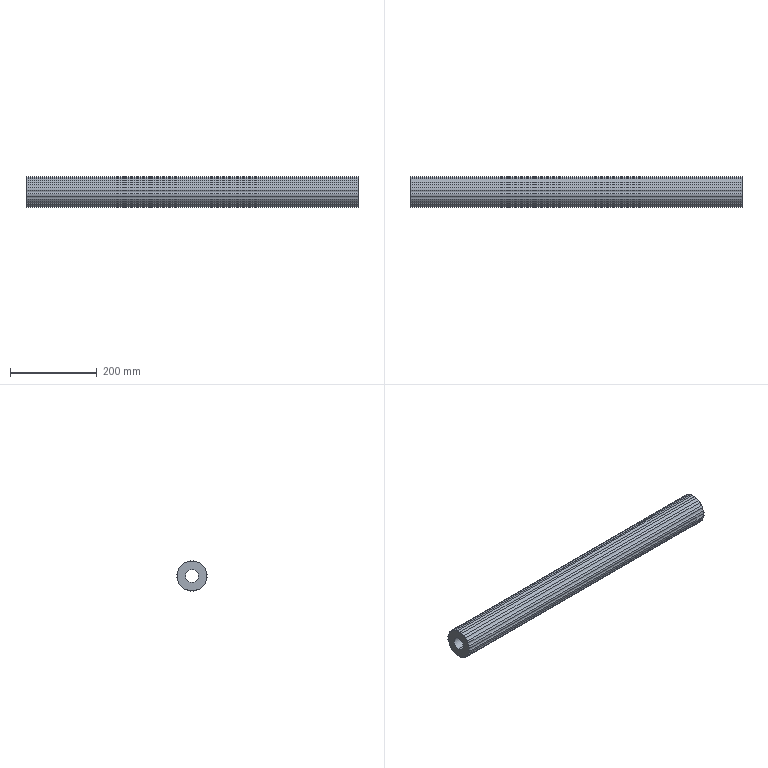Part | SolidWorks | features CirPattern 1, Extrusion 1, ICE 1 | 1 solid | 39 faces | box 767 x 69.535 x 69.535 mm | volume 2311745 mm3 | cylinder 37 | plane 2 | commonest cylinder face diameters 14.407 x19 70 x16 30 x2
STEP:
#1=CARTESIAN_POINT('',(767.,-15.591,-30.436));
#2=VERTEX_POINT('',#1);
#3=CARTESIAN_POINT('',(767.,-9.585,-33.662));
#4=VERTEX_POINT('',#3);
#5=CARTESIAN_POINT('',(767.,-15.591,-37.64));
#6=DIRECTION('',(-1.,0.,0.));
#7=DIRECTION('',(0.,0.9239,-0.3827));
#8=AXIS2_PLACEMENT_3D('',#5,#6,#7);
#9=CIRCLE('',#8,7.203);
#10=EDGE_CURVE('',#2,#4,#9,.T.);
#11=ORIENTED_EDGE('',*,*,#10,.F.);
#12=CARTESIAN_POINT('',(0.,-15.591,-30.436));
#13=VERTEX_POINT('',#12);
#14=CARTESIAN_POINT('',(767.,-15.591,-30.436));
#15=DIRECTION('',(-1.,0.,0.));
#16=VECTOR('',#15,1000.);
#17=LINE('',#14,#16);
#18=EDGE_CURVE('',#2,#13,#17,.T.);
#19=ORIENTED_EDGE('',*,*,#18,.T.);
#20=CARTESIAN_POINT('',(0.,-9.585,-33.662));
#21=VERTEX_POINT('',#20);
#22=CARTESIAN_POINT('',(0.,-15.591,-37.64));
#23=DIRECTION('',(-1.,0.,0.));
#24=DIRECTION('',(0.,0.9239,-0.3827));
#25=AXIS2_PLACEMENT_3D('',#22,#23,#24);
#26=CIRCLE('',#25,7.203);
#27=EDGE_CURVE('',#13,#21,#26,.T.);
#28=ORIENTED_EDGE('',*,*,#27,.T.);
#29=CARTESIAN_POINT('',(383.5,-9.585,-33.662));
#30=DIRECTION('',(-1.,0.,0.));
#31=VECTOR('',#30,1000.);
#32=LINE('',#29,#31);
#33=EDGE_CURVE('',#4,#21,#32,.T.);
#34=ORIENTED_EDGE('',*,*,#33,.F.);
#35=EDGE_LOOP('',(#11,#19,#28,#34));
#36=FACE_OUTER_BOUND('',#35,.T.);
#37=CARTESIAN_POINT('',(767.,-15.591,-37.64));
#38=DIRECTION('',(-1.,0.,0.));
#39=DIRECTION('',(0.,0.,1.));
#40=AXIS2_PLACEMENT_3D('',#37,#38,#39);
#41=CYLINDRICAL_SURFACE('',#40,7.203);
#42=ADVANCED_FACE('',(#36),#41,.F.);
#43=CARTESIAN_POINT('',(767.,15.591,-30.436));
#44=VERTEX_POINT('',#43);
#45=CARTESIAN_POINT('',(767.,17.025,-30.58));
#46=VERTEX_POINT('',#45);
#47=CARTESIAN_POINT('',(767.,15.591,-37.64));
#48=DIRECTION('',(-1.,0.,0.));
#49=DIRECTION('',(0.,0.9239,0.3827));
#50=AXIS2_PLACEMENT_3D('',#47,#48,#49);
#51=CIRCLE('',#50,7.203);
#52=EDGE_CURVE('',#44,#46,#51,.T.);
#53=ORIENTED_EDGE('',*,*,#52,.F.);
#54=CARTESIAN_POINT('',(0.,15.591,-30.436));
#55=VERTEX_POINT('',#54);
#56=CARTESIAN_POINT('',(767.,15.591,-30.436));
#57=DIRECTION('',(-1.,0.,0.));
#58=VECTOR('',#57,1000.);
#59=LINE('',#56,#58);
#60=EDGE_CURVE('',#44,#55,#59,.T.);
#61=ORIENTED_EDGE('',*,*,#60,.T.);
#62=CARTESIAN_POINT('',(0.,17.025,-30.58));
#63=VERTEX_POINT('',#62);
#64=CARTESIAN_POINT('',(0.,15.591,-37.64));
#65=DIRECTION('',(-1.,0.,0.));
#66=DIRECTION('',(0.,0.9239,0.3827));
#67=AXIS2_PLACEMENT_3D('',#64,#65,#66);
#68=CIRCLE('',#67,7.203);
#69=EDGE_CURVE('',#55,#63,#68,.T.);
#70=ORIENTED_EDGE('',*,*,#69,.T.);
#71=CARTESIAN_POINT('',(383.5,17.025,-30.58));
#72=DIRECTION('',(-1.,0.,0.));
#73=VECTOR('',#72,1000.);
#74=LINE('',#71,#73);
#75=EDGE_CURVE('',#46,#63,#74,.T.);
#76=ORIENTED_EDGE('',*,*,#75,.F.);
#77=EDGE_LOOP('',(#53,#61,#70,#76));
#78=FACE_OUTER_BOUND('',#77,.T.);
#79=CARTESIAN_POINT('',(767.,15.591,-37.64));
#80=DIRECTION('',(-1.,0.,0.));
#81=DIRECTION('',(0.,0.,1.));
#82=AXIS2_PLACEMENT_3D('',#79,#80,#81);
#83=CYLINDRICAL_SURFACE('',#82,7.203);
#84=ADVANCED_FACE('',(#78),#83,.F.);
#85=CARTESIAN_POINT('',(767.,0.,-33.537));
#86=VERTEX_POINT('',#85);
#87=CARTESIAN_POINT('',(767.,4.026,-34.768));
#88=VERTEX_POINT('',#87);
#89=CARTESIAN_POINT('',(767.,0.,-40.741));
#90=DIRECTION('',(-1.,0.,0.));
#91=DIRECTION('',(0.,1.,0.));
#92=AXIS2_PLACEMENT_3D('',#89,#90,#91);
#93=CIRCLE('',#92,7.203);
#94=EDGE_CURVE('',#86,#88,#93,.T.);
#95=ORIENTED_EDGE('',*,*,#94,.F.);
#96=CARTESIAN_POINT('',(0.,0.,-33.537));
#97=VERTEX_POINT('',#96);
#98=CARTESIAN_POINT('',(767.,0.,-33.537));
#99=DIRECTION('',(-1.,0.,0.));
#100=VECTOR('',#99,1000.);
#101=LINE('',#98,#100);
#102=EDGE_CURVE('',#86,#97,#101,.T.);
#103=ORIENTED_EDGE('',*,*,#102,.T.);
#104=CARTESIAN_POINT('',(0.,4.026,-34.768));
#105=VERTEX_POINT('',#104);
#106=CARTESIAN_POINT('',(0.,0.,-40.741));
#107=DIRECTION('',(-1.,0.,0.));
#108=DIRECTION('',(0.,1.,0.));
#109=AXIS2_PLACEMENT_3D('',#106,#107,#108);
#110=CIRCLE('',#109,7.203);
#111=EDGE_CURVE('',#97,#105,#110,.T.);
#112=ORIENTED_EDGE('',*,*,#111,.T.);
#113=CARTESIAN_POINT('',(383.5,4.026,-34.768));
#114=DIRECTION('',(-1.,0.,0.));
#115=VECTOR('',#114,1000.);
#116=LINE('',#113,#115);
#117=EDGE_CURVE('',#88,#105,#116,.T.);
#118=ORIENTED_EDGE('',*,*,#117,.F.);
#119=EDGE_LOOP('',(#95,#103,#112,#118));
#120=FACE_OUTER_BOUND('',#119,.T.);
#121=CARTESIAN_POINT('',(767.,0.,-40.741));
#122=DIRECTION('',(-1.,0.,0.));
#123=DIRECTION('',(0.,0.,1.));
#124=AXIS2_PLACEMENT_3D('',#121,#122,#123);
#125=CYLINDRICAL_SURFACE('',#124,7.203);
#126=ADVANCED_FACE('',(#120),#125,.F.);
#127=CARTESIAN_POINT('',(767.,0.,15.));
#128=VERTEX_POINT('',#127);
#129=CARTESIAN_POINT('',(767.,0.,-15.));
#130=VERTEX_POINT('',#129);
#131=CARTESIAN_POINT('',(767.,0.,0.));
#132=DIRECTION('',(1.,0.,0.));
#133=DIRECTION('',(0.,0.,-1.));
#134=AXIS2_PLACEMENT_3D('',#131,#132,#133);
#135=CIRCLE('',#134,15.);
#136=EDGE_CURVE('',#128,#130,#135,.T.);
#137=ORIENTED_EDGE('',*,*,#136,.T.);
#138=CARTESIAN_POINT('',(0.,0.,-15.));
#139=VERTEX_POINT('',#138);
#140=CARTESIAN_POINT('',(767.,0.,-15.));
#141=DIRECTION('',(-1.,0.,0.));
#142=VECTOR('',#141,1000.);
#143=LINE('',#140,#142);
#144=EDGE_CURVE('',#130,#139,#143,.T.);
#145=ORIENTED_EDGE('',*,*,#144,.T.);
#146=CARTESIAN_POINT('',(0.,0.,15.));
#147=VERTEX_POINT('',#146);
#148=CARTESIAN_POINT('',(0.,0.,0.));
#149=DIRECTION('',(1.,0.,0.));
#150=DIRECTION('',(0.,0.,-1.));
#151=AXIS2_PLACEMENT_3D('',#148,#149,#150);
#152=CIRCLE('',#151,15.);
#153=EDGE_CURVE('',#147,#139,#152,.T.);
#154=ORIENTED_EDGE('',*,*,#153,.F.);
#155=CARTESIAN_POINT('',(767.,0.,15.));
#156=DIRECTION('',(-1.,0.,0.));
#157=VECTOR('',#156,1000.);
#158=LINE('',#155,#157);
#159=EDGE_CURVE('',#128,#147,#158,.T.);
#160=ORIENTED_EDGE('',*,*,#159,.F.);
#161=EDGE_LOOP('',(#137,#145,#154,#160));
#162=FACE_OUTER_BOUND('',#161,.T.);
#163=CARTESIAN_POINT('',(767.,0.,0.));
#164=DIRECTION('',(-1.,0.,0.));
#165=DIRECTION('',(0.,0.,1.));
#166=AXIS2_PLACEMENT_3D('',#163,#164,#165);
#167=CYLINDRICAL_SURFACE('',#166,15.);
#168=ADVANCED_FACE('',(#162),#167,.F.);
#169=CARTESIAN_POINT('',(0.,9.585,33.662));
#170=VERTEX_POINT('',#169);
#171=CARTESIAN_POINT('',(0.,4.026,34.768));
#172=VERTEX_POINT('',#171);
#173=CARTESIAN_POINT('',(0.,0.,0.));
#174=DIRECTION('',(1.,0.,0.));
#175=DIRECTION('',(0.,0.,-1.));
#176=AXIS2_PLACEMENT_3D('',#173,#174,#175);
#177=CIRCLE('',#176,35.);
#178=EDGE_CURVE('',#170,#172,#177,.T.);
#179=ORIENTED_EDGE('',*,*,#178,.T.);
#180=CARTESIAN_POINT('',(767.,4.026,34.768));
#181=VERTEX_POINT('',#180);
#182=CARTESIAN_POINT('',(383.5,4.026,34.768));
#183=DIRECTION('',(1.,0.,0.));
#184=VECTOR('',#183,1000.);
#185=LINE('',#182,#184);
#186=EDGE_CURVE('',#172,#181,#185,.T.);
#187=ORIENTED_EDGE('',*,*,#186,.T.);
#188=CARTESIAN_POINT('',(767.,9.585,33.662));
#189=VERTEX_POINT('',#188);
#190=CARTESIAN_POINT('',(767.,0.,0.));
#191=DIRECTION('',(1.,0.,0.));
#192=DIRECTION('',(0.,0.,-1.));
#193=AXIS2_PLACEMENT_3D('',#190,#191,#192);
#194=CIRCLE('',#193,35.);
#195=EDGE_CURVE('',#189,#181,#194,.T.);
#196=ORIENTED_EDGE('',*,*,#195,.F.);
#197=CARTESIAN_POINT('',(383.5,9.585,33.662));
#198=DIRECTION('',(-1.,0.,0.));
#199=VECTOR('',#198,1000.);
#200=LINE('',#197,#199);
#201=EDGE_CURVE('',#189,#170,#200,.T.);
#202=ORIENTED_EDGE('',*,*,#201,.T.);
#203=EDGE_LOOP('',(#179,#187,#196,#202));
#204=FACE_OUTER_BOUND('',#203,.T.);
#205=CARTESIAN_POINT('',(767.,0.,0.));
#206=DIRECTION('',(-1.,0.,0.));
#207=DIRECTION('',(0.,0.,1.));
#208=AXIS2_PLACEMENT_3D('',#205,#206,#207);
#209=CYLINDRICAL_SURFACE('',#208,35.);
#210=ADVANCED_FACE('',(#204),#209,.T.);
#211=CARTESIAN_POINT('',(0.,21.737,27.431));
#212=VERTEX_POINT('',#211);
#213=CARTESIAN_POINT('',(0.,17.025,30.58));
#214=VERTEX_POINT('',#213);
#215=CARTESIAN_POINT('',(0.,0.,0.));
#216=DIRECTION('',(1.,0.,0.));
#217=DIRECTION('',(0.,0.,-1.));
#218=AXIS2_PLACEMENT_3D('',#215,#216,#217);
#219=CIRCLE('',#218,35.);
#220=EDGE_CURVE('',#212,#214,#219,.T.);
#221=ORIENTED_EDGE('',*,*,#220,.T.);
#222=CARTESIAN_POINT('',(767.,17.025,30.58));
#223=VERTEX_POINT('',#222);
#224=CARTESIAN_POINT('',(383.5,17.025,30.58));
#225=DIRECTION('',(1.,0.,0.));
#226=VECTOR('',#225,1000.);
#227=LINE('',#224,#226);
#228=EDGE_CURVE('',#214,#223,#227,.T.);
#229=ORIENTED_EDGE('',*,*,#228,.T.);
#230=CARTESIAN_POINT('',(767.,21.737,27.431));
#231=VERTEX_POINT('',#230);
#232=CARTESIAN_POINT('',(767.,0.,0.));
#233=DIRECTION('',(1.,0.,0.));
#234=DIRECTION('',(0.,0.,-1.));
#235=AXIS2_PLACEMENT_3D('',#232,#233,#234);
#236=CIRCLE('',#235,35.);
#237=EDGE_CURVE('',#231,#223,#236,.T.);
#238=ORIENTED_EDGE('',*,*,#237,.F.);
#239=CARTESIAN_POINT('',(383.5,21.737,27.431));
#240=DIRECTION('',(-1.,0.,0.));
#241=VECTOR('',#240,1000.);
#242=LINE('',#239,#241);
#243=EDGE_CURVE('',#231,#212,#242,.T.);
#244=ORIENTED_EDGE('',*,*,#243,.T.);
#245=EDGE_LOOP('',(#221,#229,#238,#244));
#246=FACE_OUTER_BOUND('',#245,.T.);
#247=CARTESIAN_POINT('',(767.,0.,0.));
#248=DIRECTION('',(-1.,0.,0.));
#249=DIRECTION('',(0.,0.,1.));
#250=AXIS2_PLACEMENT_3D('',#247,#248,#249);
#251=CYLINDRICAL_SURFACE('',#250,35.);
#252=ADVANCED_FACE('',(#246),#251,.T.);
#253=CARTESIAN_POINT('',(0.,30.58,17.025));
#254=VERTEX_POINT('',#253);
#255=CARTESIAN_POINT('',(0.,27.431,21.737));
#256=VERTEX_POINT('',#255);
#257=CARTESIAN_POINT('',(0.,0.,0.));
#258=DIRECTION('',(1.,0.,0.));
#259=DIRECTION('',(0.,0.,-1.));
#260=AXIS2_PLACEMENT_3D('',#257,#258,#259);
#261=CIRCLE('',#260,35.);
#262=EDGE_CURVE('',#254,#256,#261,.T.);
#263=ORIENTED_EDGE('',*,*,#262,.T.);
#264=CARTESIAN_POINT('',(767.,27.431,21.737));
#265=VERTEX_POINT('',#264);
#266=CARTESIAN_POINT('',(383.5,27.431,21.737));
#267=DIRECTION('',(1.,0.,0.));
#268=VECTOR('',#267,1000.);
#269=LINE('',#266,#268);
#270=EDGE_CURVE('',#256,#265,#269,.T.);
#271=ORIENTED_EDGE('',*,*,#270,.T.);
#272=CARTESIAN_POINT('',(767.,30.58,17.025));
#273=VERTEX_POINT('',#272);
#274=CARTESIAN_POINT('',(767.,0.,0.));
#275=DIRECTION('',(1.,0.,0.));
#276=DIRECTION('',(0.,0.,-1.));
#277=AXIS2_PLACEMENT_3D('',#274,#275,#276);
#278=CIRCLE('',#277,35.);
#279=EDGE_CURVE('',#273,#265,#278,.T.);
#280=ORIENTED_EDGE('',*,*,#279,.F.);
#281=CARTESIAN_POINT('',(383.5,30.58,17.025));
#282=DIRECTION('',(-1.,0.,0.));
#283=VECTOR('',#282,1000.);
#284=LINE('',#281,#283);
#285=EDGE_CURVE('',#273,#254,#284,.T.);
#286=ORIENTED_EDGE('',*,*,#285,.T.);
#287=EDGE_LOOP('',(#263,#271,#280,#286));
#288=FACE_OUTER_BOUND('',#287,.T.);
#289=CARTESIAN_POINT('',(767.,0.,0.));
#290=DIRECTION('',(-1.,0.,0.));
#291=DIRECTION('',(0.,0.,1.));
#292=AXIS2_PLACEMENT_3D('',#289,#290,#291);
#293=CYLINDRICAL_SURFACE('',#292,35.);
#294=ADVANCED_FACE('',(#288),#293,.T.);
#295=CARTESIAN_POINT('',(0.,-33.662,9.585));
#296=VERTEX_POINT('',#295);
#297=CARTESIAN_POINT('',(0.,-34.768,4.026));
#298=VERTEX_POINT('',#297);
#299=CARTESIAN_POINT('',(0.,0.,0.));
#300=DIRECTION('',(1.,0.,0.));
#301=DIRECTION('',(0.,0.,-1.));
#302=AXIS2_PLACEMENT_3D('',#299,#300,#301);
#303=CIRCLE('',#302,35.);
#304=EDGE_CURVE('',#296,#298,#303,.T.);
#305=ORIENTED_EDGE('',*,*,#304,.T.);
#306=CARTESIAN_POINT('',(767.,-34.768,4.026));
#307=VERTEX_POINT('',#306);
#308=CARTESIAN_POINT('',(383.5,-34.768,4.026));
#309=DIRECTION('',(1.,0.,0.));
#310=VECTOR('',#309,1000.);
#311=LINE('',#308,#310);
#312=EDGE_CURVE('',#298,#307,#311,.T.);
#313=ORIENTED_EDGE('',*,*,#312,.T.);
#314=CARTESIAN_POINT('',(767.,-33.662,9.585));
#315=VERTEX_POINT('',#314);
#316=CARTESIAN_POINT('',(767.,0.,0.));
#317=DIRECTION('',(1.,0.,0.));
#318=DIRECTION('',(0.,0.,-1.));
#319=AXIS2_PLACEMENT_3D('',#316,#317,#318);
#320=CIRCLE('',#319,35.);
#321=EDGE_CURVE('',#315,#307,#320,.T.);
#322=ORIENTED_EDGE('',*,*,#321,.F.);
#323=CARTESIAN_POINT('',(383.5,-33.662,9.585));
#324=DIRECTION('',(-1.,0.,0.));
#325=VECTOR('',#324,1000.);
#326=LINE('',#323,#325);
#327=EDGE_CURVE('',#315,#296,#326,.T.);
#328=ORIENTED_EDGE('',*,*,#327,.T.);
#329=EDGE_LOOP('',(#305,#313,#322,#328));
#330=FACE_OUTER_BOUND('',#329,.T.);
#331=CARTESIAN_POINT('',(767.,0.,0.));
#332=DIRECTION('',(-1.,0.,0.));
#333=DIRECTION('',(0.,0.,1.));
#334=AXIS2_PLACEMENT_3D('',#331,#332,#333);
#335=CYLINDRICAL_SURFACE('',#334,35.);
#336=ADVANCED_FACE('',(#330),#335,.T.);
#337=CARTESIAN_POINT('',(0.,-27.431,21.737));
#338=VERTEX_POINT('',#337);
#339=CARTESIAN_POINT('',(0.,-30.58,17.025));
#340=VERTEX_POINT('',#339);
#341=CARTESIAN_POINT('',(0.,0.,0.));
#342=DIRECTION('',(1.,0.,0.));
#343=DIRECTION('',(0.,0.,-1.));
#344=AXIS2_PLACEMENT_3D('',#341,#342,#343);
#345=CIRCLE('',#344,35.);
#346=EDGE_CURVE('',#338,#340,#345,.T.);
#347=ORIENTED_EDGE('',*,*,#346,.T.);
#348=CARTESIAN_POINT('',(767.,-30.58,17.025));
#349=VERTEX_POINT('',#348);
#350=CARTESIAN_POINT('',(383.5,-30.58,17.025));
#351=DIRECTION('',(1.,0.,0.));
#352=VECTOR('',#351,1000.);
#353=LINE('',#350,#352);
#354=EDGE_CURVE('',#340,#349,#353,.T.);
#355=ORIENTED_EDGE('',*,*,#354,.T.);
#356=CARTESIAN_POINT('',(767.,-27.431,21.737));
#357=VERTEX_POINT('',#356);
#358=CARTESIAN_POINT('',(767.,0.,0.));
#359=DIRECTION('',(1.,0.,0.));
#360=DIRECTION('',(0.,0.,-1.));
#361=AXIS2_PLACEMENT_3D('',#358,#359,#360);
#362=CIRCLE('',#361,35.);
#363=EDGE_CURVE('',#357,#349,#362,.T.);
#364=ORIENTED_EDGE('',*,*,#363,.F.);
#365=CARTESIAN_POINT('',(383.5,-27.431,21.737));
#366=DIRECTION('',(-1.,0.,0.));
#367=VECTOR('',#366,1000.);
#368=LINE('',#365,#367);
#369=EDGE_CURVE('',#357,#338,#368,.T.);
#370=ORIENTED_EDGE('',*,*,#369,.T.);
#371=EDGE_LOOP('',(#347,#355,#364,#370));
#372=FACE_OUTER_BOUND('',#371,.T.);
#373=CARTESIAN_POINT('',(767.,0.,0.));
#374=DIRECTION('',(-1.,0.,0.));
#375=DIRECTION('',(0.,0.,1.));
#376=AXIS2_PLACEMENT_3D('',#373,#374,#375);
#377=CYLINDRICAL_SURFACE('',#376,35.);
#378=ADVANCED_FACE('',(#372),#377,.T.);
#379=CARTESIAN_POINT('',(767.,-4.026,34.768));
#380=VERTEX_POINT('',#379);
#381=CARTESIAN_POINT('',(767.,-9.585,33.662));
#382=VERTEX_POINT('',#381);
#383=CARTESIAN_POINT('',(767.,0.,0.));
#384=DIRECTION('',(1.,0.,0.));
#385=DIRECTION('',(0.,0.,-1.));
#386=AXIS2_PLACEMENT_3D('',#383,#384,#385);
#387=CIRCLE('',#386,35.);
#388=EDGE_CURVE('',#380,#382,#387,.T.);
#389=ORIENTED_EDGE('',*,*,#388,.F.);
#390=CARTESIAN_POINT('',(0.,-4.026,34.768));
#391=VERTEX_POINT('',#390);
#392=CARTESIAN_POINT('',(383.5,-4.026,34.768));
#393=DIRECTION('',(-1.,0.,0.));
#394=VECTOR('',#393,1000.);
#395=LINE('',#392,#394);
#396=EDGE_CURVE('',#380,#391,#395,.T.);
#397=ORIENTED_EDGE('',*,*,#396,.T.);
#398=CARTESIAN_POINT('',(0.,-9.585,33.662));
#399=VERTEX_POINT('',#398);
#400=CARTESIAN_POINT('',(0.,0.,0.));
#401=DIRECTION('',(1.,0.,0.));
#402=DIRECTION('',(0.,0.,-1.));
#403=AXIS2_PLACEMENT_3D('',#400,#401,#402);
#404=CIRCLE('',#403,35.);
#405=EDGE_CURVE('',#391,#399,#404,.T.);
#406=ORIENTED_EDGE('',*,*,#405,.T.);
#407=CARTESIAN_POINT('',(383.5,-9.585,33.662));
#408=DIRECTION('',(1.,0.,0.));
#409=VECTOR('',#408,1000.);
#410=LINE('',#407,#409);
#411=EDGE_CURVE('',#399,#382,#410,.T.);
#412=ORIENTED_EDGE('',*,*,#411,.T.);
#413=EDGE_LOOP('',(#389,#397,#406,#412));
#414=FACE_OUTER_BOUND('',#413,.T.);
#415=CARTESIAN_POINT('',(767.,0.,0.));
#416=DIRECTION('',(-1.,0.,0.));
#417=DIRECTION('',(0.,0.,1.));
#418=AXIS2_PLACEMENT_3D('',#415,#416,#417);
#419=CYLINDRICAL_SURFACE('',#418,35.);
#420=ADVANCED_FACE('',(#414),#419,.T.);
#421=CARTESIAN_POINT('',(767.,-17.025,30.58));
#422=VERTEX_POINT('',#421);
#423=CARTESIAN_POINT('',(767.,-21.737,27.431));
#424=VERTEX_POINT('',#423);
#425=CARTESIAN_POINT('',(767.,0.,0.));
#426=DIRECTION('',(1.,0.,0.));
#427=DIRECTION('',(0.,0.,-1.));
#428=AXIS2_PLACEMENT_3D('',#425,#426,#427);
#429=CIRCLE('',#428,35.);
#430=EDGE_CURVE('',#422,#424,#429,.T.);
#431=ORIENTED_EDGE('',*,*,#430,.F.);
#432=CARTESIAN_POINT('',(0.,-17.025,30.58));
#433=VERTEX_POINT('',#432);
#434=CARTESIAN_POINT('',(383.5,-17.025,30.58));
#435=DIRECTION('',(-1.,0.,0.));
#436=VECTOR('',#435,1000.);
#437=LINE('',#434,#436);
#438=EDGE_CURVE('',#422,#433,#437,.T.);
#439=ORIENTED_EDGE('',*,*,#438,.T.);
#440=CARTESIAN_POINT('',(0.,-21.737,27.431));
#441=VERTEX_POINT('',#440);
#442=CARTESIAN_POINT('',(0.,0.,0.));
#443=DIRECTION('',(1.,0.,0.));
#444=DIRECTION('',(0.,0.,-1.));
#445=AXIS2_PLACEMENT_3D('',#442,#443,#444);
#446=CIRCLE('',#445,35.);
#447=EDGE_CURVE('',#433,#441,#446,.T.);
#448=ORIENTED_EDGE('',*,*,#447,.T.);
#449=CARTESIAN_POINT('',(383.5,-21.737,27.431));
#450=DIRECTION('',(1.,0.,0.));
#451=VECTOR('',#450,1000.);
#452=LINE('',#449,#451);
#453=EDGE_CURVE('',#441,#424,#452,.T.);
#454=ORIENTED_EDGE('',*,*,#453,.T.);
#455=EDGE_LOOP('',(#431,#439,#448,#454));
#456=FACE_OUTER_BOUND('',#455,.T.);
#457=CARTESIAN_POINT('',(767.,0.,0.));
#458=DIRECTION('',(-1.,0.,0.));
#459=DIRECTION('',(0.,0.,1.));
#460=AXIS2_PLACEMENT_3D('',#457,#458,#459);
#461=CYLINDRICAL_SURFACE('',#460,35.);
#462=ADVANCED_FACE('',(#456),#461,.T.);
#463=CARTESIAN_POINT('',(0.,-30.58,-17.025));
#464=VERTEX_POINT('',#463);
#465=CARTESIAN_POINT('',(0.,-27.431,-21.737));
#466=VERTEX_POINT('',#465);
#467=CARTESIAN_POINT('',(0.,0.,0.));
#468=DIRECTION('',(1.,0.,0.));
#469=DIRECTION('',(0.,0.,-1.));
#470=AXIS2_PLACEMENT_3D('',#467,#468,#469);
#471=CIRCLE('',#470,35.);
#472=EDGE_CURVE('',#464,#466,#471,.T.);
#473=ORIENTED_EDGE('',*,*,#472,.T.);
#474=CARTESIAN_POINT('',(767.,-27.431,-21.737));
#475=VERTEX_POINT('',#474);
#476=CARTESIAN_POINT('',(383.5,-27.431,-21.737));
#477=DIRECTION('',(1.,0.,0.));
#478=VECTOR('',#477,1000.);
#479=LINE('',#476,#478);
#480=EDGE_CURVE('',#466,#475,#479,.T.);
#481=ORIENTED_EDGE('',*,*,#480,.T.);
#482=CARTESIAN_POINT('',(767.,-30.58,-17.025));
#483=VERTEX_POINT('',#482);
#484=CARTESIAN_POINT('',(767.,0.,0.));
#485=DIRECTION('',(1.,0.,0.));
#486=DIRECTION('',(0.,0.,-1.));
#487=AXIS2_PLACEMENT_3D('',#484,#485,#486);
#488=CIRCLE('',#487,35.);
#489=EDGE_CURVE('',#483,#475,#488,.T.);
#490=ORIENTED_EDGE('',*,*,#489,.F.);
#491=CARTESIAN_POINT('',(383.5,-30.58,-17.025));
#492=DIRECTION('',(-1.,0.,0.));
#493=VECTOR('',#492,1000.);
#494=LINE('',#491,#493);
#495=EDGE_CURVE('',#483,#464,#494,.T.);
#496=ORIENTED_EDGE('',*,*,#495,.T.);
#497=EDGE_LOOP('',(#473,#481,#490,#496));
#498=FACE_OUTER_BOUND('',#497,.T.);
#499=CARTESIAN_POINT('',(767.,0.,0.));
#500=DIRECTION('',(-1.,0.,0.));
#501=DIRECTION('',(0.,0.,1.));
#502=AXIS2_PLACEMENT_3D('',#499,#500,#501);
#503=CYLINDRICAL_SURFACE('',#502,35.);
#504=ADVANCED_FACE('',(#498),#503,.T.);
#505=CARTESIAN_POINT('',(767.,-21.737,-27.431));
#506=VERTEX_POINT('',#505);
#507=CARTESIAN_POINT('',(767.,-17.025,-30.58));
#508=VERTEX_POINT('',#507);
#509=CARTESIAN_POINT('',(767.,0.,0.));
#510=DIRECTION('',(1.,0.,0.));
#511=DIRECTION('',(0.,0.,-1.));
#512=AXIS2_PLACEMENT_3D('',#509,#510,#511);
#513=CIRCLE('',#512,35.);
#514=EDGE_CURVE('',#506,#508,#513,.T.);
#515=ORIENTED_EDGE('',*,*,#514,.F.);
#516=CARTESIAN_POINT('',(0.,-21.737,-27.431));
#517=VERTEX_POINT('',#516);
#518=CARTESIAN_POINT('',(383.5,-21.737,-27.431));
#519=DIRECTION('',(-1.,0.,0.));
#520=VECTOR('',#519,1000.);
#521=LINE('',#518,#520);
#522=EDGE_CURVE('',#506,#517,#521,.T.);
#523=ORIENTED_EDGE('',*,*,#522,.T.);
#524=CARTESIAN_POINT('',(0.,-17.025,-30.58));
#525=VERTEX_POINT('',#524);
#526=CARTESIAN_POINT('',(0.,0.,0.));
#527=DIRECTION('',(1.,0.,0.));
#528=DIRECTION('',(0.,0.,-1.));
#529=AXIS2_PLACEMENT_3D('',#526,#527,#528);
#530=CIRCLE('',#529,35.);
#531=EDGE_CURVE('',#517,#525,#530,.T.);
#532=ORIENTED_EDGE('',*,*,#531,.T.);
#533=CARTESIAN_POINT('',(383.5,-17.025,-30.58));
#534=DIRECTION('',(1.,0.,0.));
#535=VECTOR('',#534,1000.);
#536=LINE('',#533,#535);
#537=EDGE_CURVE('',#525,#508,#536,.T.);
#538=ORIENTED_EDGE('',*,*,#537,.T.);
#539=EDGE_LOOP('',(#515,#523,#532,#538));
#540=FACE_OUTER_BOUND('',#539,.T.);
#541=CARTESIAN_POINT('',(767.,0.,0.));
#542=DIRECTION('',(-1.,0.,0.));
#543=DIRECTION('',(0.,0.,1.));
#544=AXIS2_PLACEMENT_3D('',#541,#542,#543);
#545=CYLINDRICAL_SURFACE('',#544,35.);
#546=ADVANCED_FACE('',(#540),#545,.T.);
#547=CARTESIAN_POINT('',(767.,-34.768,-4.026));
#548=VERTEX_POINT('',#547);
#549=CARTESIAN_POINT('',(767.,-33.662,-9.585));
#550=VERTEX_POINT('',#549);
#551=CARTESIAN_POINT('',(767.,0.,0.));
#552=DIRECTION('',(1.,0.,0.));
#553=DIRECTION('',(0.,0.,-1.));
#554=AXIS2_PLACEMENT_3D('',#551,#552,#553);
#555=CIRCLE('',#554,35.);
#556=EDGE_CURVE('',#548,#550,#555,.T.);
#557=ORIENTED_EDGE('',*,*,#556,.F.);
#558=CARTESIAN_POINT('',(0.,-34.768,-4.026));
#559=VERTEX_POINT('',#558);
#560=CARTESIAN_POINT('',(383.5,-34.768,-4.026));
#561=DIRECTION('',(-1.,0.,0.));
#562=VECTOR('',#561,1000.);
#563=LINE('',#560,#562);
#564=EDGE_CURVE('',#548,#559,#563,.T.);
#565=ORIENTED_EDGE('',*,*,#564,.T.);
#566=CARTESIAN_POINT('',(0.,-33.662,-9.585));
#567=VERTEX_POINT('',#566);
#568=CARTESIAN_POINT('',(0.,0.,0.));
#569=DIRECTION('',(1.,0.,0.));
#570=DIRECTION('',(0.,0.,-1.));
#571=AXIS2_PLACEMENT_3D('',#568,#569,#570);
#572=CIRCLE('',#571,35.);
#573=EDGE_CURVE('',#559,#567,#572,.T.);
#574=ORIENTED_EDGE('',*,*,#573,.T.);
#575=CARTESIAN_POINT('',(383.5,-33.662,-9.585));
#576=DIRECTION('',(1.,0.,0.));
#577=VECTOR('',#576,1000.);
#578=LINE('',#575,#577);
#579=EDGE_CURVE('',#567,#550,#578,.T.);
#580=ORIENTED_EDGE('',*,*,#579,.T.);
#581=EDGE_LOOP('',(#557,#565,#574,#580));
#582=FACE_OUTER_BOUND('',#581,.T.);
#583=CARTESIAN_POINT('',(767.,0.,0.));
#584=DIRECTION('',(-1.,0.,0.));
#585=DIRECTION('',(0.,0.,1.));
#586=AXIS2_PLACEMENT_3D('',#583,#584,#585);
#587=CYLINDRICAL_SURFACE('',#586,35.);
#588=ADVANCED_FACE('',(#582),#587,.T.);
#589=CARTESIAN_POINT('',(0.,21.737,-27.431));
#590=VERTEX_POINT('',#589);
#591=CARTESIAN_POINT('',(0.,0.,0.));
#592=DIRECTION('',(1.,0.,0.));
#593=DIRECTION('',(0.,0.,-1.));
#594=AXIS2_PLACEMENT_3D('',#591,#592,#593);
#595=CIRCLE('',#594,35.);
#596=EDGE_CURVE('',#63,#590,#595,.T.);
#597=ORIENTED_EDGE('',*,*,#596,.T.);
#598=CARTESIAN_POINT('',(767.,21.737,-27.431));
#599=VERTEX_POINT('',#598);
#600=CARTESIAN_POINT('',(383.5,21.737,-27.431));
#601=DIRECTION('',(1.,0.,0.));
#602=VECTOR('',#601,1000.);
#603=LINE('',#600,#602);
#604=EDGE_CURVE('',#590,#599,#603,.T.);
#605=ORIENTED_EDGE('',*,*,#604,.T.);
#606=CARTESIAN_POINT('',(767.,0.,0.));
#607=DIRECTION('',(1.,0.,0.));
#608=DIRECTION('',(0.,0.,-1.));
#609=AXIS2_PLACEMENT_3D('',#606,#607,#608);
#610=CIRCLE('',#609,35.);
#611=EDGE_CURVE('',#46,#599,#610,.T.);
#612=ORIENTED_EDGE('',*,*,#611,.F.);
#613=ORIENTED_EDGE('',*,*,#75,.T.);
#614=EDGE_LOOP('',(#597,#605,#612,#613));
#615=FACE_OUTER_BOUND('',#614,.T.);
#616=CARTESIAN_POINT('',(767.,0.,0.));
#617=DIRECTION('',(-1.,0.,0.));
#618=DIRECTION('',(0.,0.,1.));
#619=AXIS2_PLACEMENT_3D('',#616,#617,#618);
#620=CYLINDRICAL_SURFACE('',#619,35.);
#621=ADVANCED_FACE('',(#615),#620,.T.);
#622=CARTESIAN_POINT('',(767.,27.431,-21.737));
#623=VERTEX_POINT('',#622);
#624=CARTESIAN_POINT('',(767.,30.58,-17.025));
#625=VERTEX_POINT('',#624);
#626=CARTESIAN_POINT('',(767.,0.,0.));
#627=DIRECTION('',(1.,0.,0.));
#628=DIRECTION('',(0.,0.,-1.));
#629=AXIS2_PLACEMENT_3D('',#626,#627,#628);
#630=CIRCLE('',#629,35.);
#631=EDGE_CURVE('',#623,#625,#630,.T.);
#632=ORIENTED_EDGE('',*,*,#631,.F.);
#633=CARTESIAN_POINT('',(0.,27.431,-21.737));
#634=VERTEX_POINT('',#633);
#635=CARTESIAN_POINT('',(383.5,27.431,-21.737));
#636=DIRECTION('',(-1.,0.,0.));
#637=VECTOR('',#636,1000.);
#638=LINE('',#635,#637);
#639=EDGE_CURVE('',#623,#634,#638,.T.);
#640=ORIENTED_EDGE('',*,*,#639,.T.);
#641=CARTESIAN_POINT('',(0.,30.58,-17.025));
#642=VERTEX_POINT('',#641);
#643=CARTESIAN_POINT('',(0.,0.,0.));
#644=DIRECTION('',(1.,0.,0.));
#645=DIRECTION('',(0.,0.,-1.));
#646=AXIS2_PLACEMENT_3D('',#643,#644,#645);
#647=CIRCLE('',#646,35.);
#648=EDGE_CURVE('',#634,#642,#647,.T.);
#649=ORIENTED_EDGE('',*,*,#648,.T.);
#650=CARTESIAN_POINT('',(383.5,30.58,-17.025));
#651=DIRECTION('',(1.,0.,0.));
#652=VECTOR('',#651,1000.);
#653=LINE('',#650,#652);
#654=EDGE_CURVE('',#642,#625,#653,.T.);
#655=ORIENTED_EDGE('',*,*,#654,.T.);
#656=EDGE_LOOP('',(#632,#640,#649,#655));
#657=FACE_OUTER_BOUND('',#656,.T.);
#658=CARTESIAN_POINT('',(767.,0.,0.));
#659=DIRECTION('',(-1.,0.,0.));
#660=DIRECTION('',(0.,0.,1.));
#661=AXIS2_PLACEMENT_3D('',#658,#659,#660);
#662=CYLINDRICAL_SURFACE('',#661,35.);
#663=ADVANCED_FACE('',(#657),#662,.T.);
#664=CARTESIAN_POINT('',(0.,9.585,-33.662));
#665=VERTEX_POINT('',#664);
#666=CARTESIAN_POINT('',(0.,0.,0.));
#667=DIRECTION('',(1.,0.,0.));
#668=DIRECTION('',(0.,0.,-1.));
#669=AXIS2_PLACEMENT_3D('',#666,#667,#668);
#670=CIRCLE('',#669,35.);
#671=EDGE_CURVE('',#105,#665,#670,.T.);
#672=ORIENTED_EDGE('',*,*,#671,.T.);
#673=CARTESIAN_POINT('',(767.,9.585,-33.662));
#674=VERTEX_POINT('',#673);
#675=CARTESIAN_POINT('',(383.5,9.585,-33.662));
#676=DIRECTION('',(1.,0.,0.));
#677=VECTOR('',#676,1000.);
#678=LINE('',#675,#677);
#679=EDGE_CURVE('',#665,#674,#678,.T.);
#680=ORIENTED_EDGE('',*,*,#679,.T.);
#681=CARTESIAN_POINT('',(767.,0.,0.));
#682=DIRECTION('',(1.,0.,0.));
#683=DIRECTION('',(0.,0.,-1.));
#684=AXIS2_PLACEMENT_3D('',#681,#682,#683);
#685=CIRCLE('',#684,35.);
#686=EDGE_CURVE('',#88,#674,#685,.T.);
#687=ORIENTED_EDGE('',*,*,#686,.F.);
#688=ORIENTED_EDGE('',*,*,#117,.T.);
#689=EDGE_LOOP('',(#672,#680,#687,#688));
#690=FACE_OUTER_BOUND('',#689,.T.);
#691=CARTESIAN_POINT('',(767.,0.,0.));
#692=DIRECTION('',(-1.,0.,0.));
#693=DIRECTION('',(0.,0.,1.));
#694=AXIS2_PLACEMENT_3D('',#691,#692,#693);
#695=CYLINDRICAL_SURFACE('',#694,35.);
#696=ADVANCED_FACE('',(#690),#695,.T.);
#697=CARTESIAN_POINT('',(767.,-4.026,-34.768));
#698=VERTEX_POINT('',#697);
#699=CARTESIAN_POINT('',(767.,0.,0.));
#700=DIRECTION('',(1.,0.,0.));
#701=DIRECTION('',(0.,0.,-1.));
#702=AXIS2_PLACEMENT_3D('',#699,#700,#701);
#703=CIRCLE('',#702,35.);
#704=EDGE_CURVE('',#4,#698,#703,.T.);
#705=ORIENTED_EDGE('',*,*,#704,.F.);
#706=ORIENTED_EDGE('',*,*,#33,.T.);
#707=CARTESIAN_POINT('',(0.,-4.026,-34.768));
#708=VERTEX_POINT('',#707);
#709=CARTESIAN_POINT('',(0.,0.,0.));
#710=DIRECTION('',(1.,0.,0.));
#711=DIRECTION('',(0.,0.,-1.));
#712=AXIS2_PLACEMENT_3D('',#709,#710,#711);
#713=CIRCLE('',#712,35.);
#714=EDGE_CURVE('',#21,#708,#713,.T.);
#715=ORIENTED_EDGE('',*,*,#714,.T.);
#716=CARTESIAN_POINT('',(383.5,-4.026,-34.768));
#717=DIRECTION('',(1.,0.,0.));
#718=VECTOR('',#717,1000.);
#719=LINE('',#716,#718);
#720=EDGE_CURVE('',#708,#698,#719,.T.);
#721=ORIENTED_EDGE('',*,*,#720,.T.);
#722=EDGE_LOOP('',(#705,#706,#715,#721));
#723=FACE_OUTER_BOUND('',#722,.T.);
#724=CARTESIAN_POINT('',(767.,0.,0.));
#725=DIRECTION('',(-1.,0.,0.));
#726=DIRECTION('',(0.,0.,1.));
#727=AXIS2_PLACEMENT_3D('',#724,#725,#726);
#728=CYLINDRICAL_SURFACE('',#727,35.);
#729=ADVANCED_FACE('',(#723),#728,.T.);
#730=CARTESIAN_POINT('',(0.,34.768,4.026));
#731=VERTEX_POINT('',#730);
#732=CARTESIAN_POINT('',(0.,33.662,9.585));
#733=VERTEX_POINT('',#732);
#734=CARTESIAN_POINT('',(0.,0.,0.));
#735=DIRECTION('',(1.,0.,0.));
#736=DIRECTION('',(0.,0.,-1.));
#737=AXIS2_PLACEMENT_3D('',#734,#735,#736);
#738=CIRCLE('',#737,35.);
#739=EDGE_CURVE('',#731,#733,#738,.T.);
#740=ORIENTED_EDGE('',*,*,#739,.T.);
#741=CARTESIAN_POINT('',(767.,33.662,9.585));
#742=VERTEX_POINT('',#741);
#743=CARTESIAN_POINT('',(383.5,33.662,9.585));
#744=DIRECTION('',(1.,0.,0.));
#745=VECTOR('',#744,1000.);
#746=LINE('',#743,#745);
#747=EDGE_CURVE('',#733,#742,#746,.T.);
#748=ORIENTED_EDGE('',*,*,#747,.T.);
#749=CARTESIAN_POINT('',(767.,34.768,4.026));
#750=VERTEX_POINT('',#749);
#751=CARTESIAN_POINT('',(767.,0.,0.));
#752=DIRECTION('',(1.,0.,0.));
#753=DIRECTION('',(0.,0.,-1.));
#754=AXIS2_PLACEMENT_3D('',#751,#752,#753);
#755=CIRCLE('',#754,35.);
#756=EDGE_CURVE('',#750,#742,#755,.T.);
#757=ORIENTED_EDGE('',*,*,#756,.F.);
#758=CARTESIAN_POINT('',(383.5,34.768,4.026));
#759=DIRECTION('',(-1.,0.,0.));
#760=VECTOR('',#759,1000.);
#761=LINE('',#758,#760);
#762=EDGE_CURVE('',#750,#731,#761,.T.);
#763=ORIENTED_EDGE('',*,*,#762,.T.);
#764=EDGE_LOOP('',(#740,#748,#757,#763));
#765=FACE_OUTER_BOUND('',#764,.T.);
#766=CARTESIAN_POINT('',(767.,0.,0.));
#767=DIRECTION('',(-1.,0.,0.));
#768=DIRECTION('',(0.,0.,1.));
#769=AXIS2_PLACEMENT_3D('',#766,#767,#768);
#770=CYLINDRICAL_SURFACE('',#769,35.);
#771=ADVANCED_FACE('',(#765),#770,.T.);
#772=CARTESIAN_POINT('',(767.,0.,40.741));
#773=DIRECTION('',(-1.,0.,0.));
#774=DIRECTION('',(0.,-1.,0.));
#775=AXIS2_PLACEMENT_3D('',#772,#773,#774);
#776=CIRCLE('',#775,7.203);
#777=EDGE_CURVE('',#181,#380,#776,.T.);
#778=ORIENTED_EDGE('',*,*,#777,.T.);
#779=ORIENTED_EDGE('',*,*,#388,.T.);
#780=CARTESIAN_POINT('',(767.,-15.591,37.64));
#781=DIRECTION('',(-1.,0.,0.));
#782=DIRECTION('',(0.,-0.9239,-0.3827));
#783=AXIS2_PLACEMENT_3D('',#780,#781,#782);
#784=CIRCLE('',#783,7.203);
#785=EDGE_CURVE('',#382,#422,#784,.T.);
#786=ORIENTED_EDGE('',*,*,#785,.T.);
#787=ORIENTED_EDGE('',*,*,#430,.T.);
#788=CARTESIAN_POINT('',(767.,-28.808,28.808));
#789=DIRECTION('',(-1.,0.,0.));
#790=DIRECTION('',(0.,-0.7071,-0.7071));
#791=AXIS2_PLACEMENT_3D('',#788,#789,#790);
#792=CIRCLE('',#791,7.203);
#793=EDGE_CURVE('',#424,#357,#792,.T.);
#794=ORIENTED_EDGE('',*,*,#793,.T.);
#795=ORIENTED_EDGE('',*,*,#363,.T.);
#796=CARTESIAN_POINT('',(767.,-37.64,15.591));
#797=DIRECTION('',(-1.,0.,0.));
#798=DIRECTION('',(0.,-0.3827,-0.9239));
#799=AXIS2_PLACEMENT_3D('',#796,#797,#798);
#800=CIRCLE('',#799,7.203);
#801=EDGE_CURVE('',#349,#315,#800,.T.);
#802=ORIENTED_EDGE('',*,*,#801,.T.);
#803=ORIENTED_EDGE('',*,*,#321,.T.);
#804=CARTESIAN_POINT('',(767.,-40.741,0.));
#805=DIRECTION('',(-1.,0.,0.));
#806=DIRECTION('',(0.,0.,-1.));
#807=AXIS2_PLACEMENT_3D('',#804,#805,#806);
#808=CIRCLE('',#807,7.203);
#809=EDGE_CURVE('',#307,#548,#808,.T.);
#810=ORIENTED_EDGE('',*,*,#809,.T.);
#811=ORIENTED_EDGE('',*,*,#556,.T.);
#812=CARTESIAN_POINT('',(767.,-37.64,-15.591));
#813=DIRECTION('',(-1.,0.,0.));
#814=DIRECTION('',(0.,0.3827,-0.9239));
#815=AXIS2_PLACEMENT_3D('',#812,#813,#814);
#816=CIRCLE('',#815,7.203);
#817=EDGE_CURVE('',#550,#483,#816,.T.);
#818=ORIENTED_EDGE('',*,*,#817,.T.);
#819=ORIENTED_EDGE('',*,*,#489,.T.);
#820=CARTESIAN_POINT('',(767.,-28.808,-28.808));
#821=DIRECTION('',(-1.,0.,0.));
#822=DIRECTION('',(0.,0.7071,-0.7071));
#823=AXIS2_PLACEMENT_3D('',#820,#821,#822);
#824=CIRCLE('',#823,7.203);
#825=EDGE_CURVE('',#475,#506,#824,.T.);
#826=ORIENTED_EDGE('',*,*,#825,.T.);
#827=ORIENTED_EDGE('',*,*,#514,.T.);
#828=CARTESIAN_POINT('',(767.,-15.591,-37.64));
#829=DIRECTION('',(-1.,0.,0.));
#830=DIRECTION('',(0.,0.9239,-0.3827));
#831=AXIS2_PLACEMENT_3D('',#828,#829,#830);
#832=CIRCLE('',#831,7.203);
#833=EDGE_CURVE('',#508,#2,#832,.T.);
#834=ORIENTED_EDGE('',*,*,#833,.T.);
#835=ORIENTED_EDGE('',*,*,#10,.T.);
#836=ORIENTED_EDGE('',*,*,#704,.T.);
#837=CARTESIAN_POINT('',(767.,0.,-40.741));
#838=DIRECTION('',(-1.,0.,0.));
#839=DIRECTION('',(0.,1.,0.));
#840=AXIS2_PLACEMENT_3D('',#837,#838,#839);
#841=CIRCLE('',#840,7.203);
#842=EDGE_CURVE('',#698,#86,#841,.T.);
#843=ORIENTED_EDGE('',*,*,#842,.T.);
#844=ORIENTED_EDGE('',*,*,#94,.T.);
#845=ORIENTED_EDGE('',*,*,#686,.T.);
#846=CARTESIAN_POINT('',(767.,15.591,-37.64));
#847=DIRECTION('',(-1.,0.,0.));
#848=DIRECTION('',(0.,0.9239,0.3827));
#849=AXIS2_PLACEMENT_3D('',#846,#847,#848);
#850=CIRCLE('',#849,7.203);
#851=EDGE_CURVE('',#674,#44,#850,.T.);
#852=ORIENTED_EDGE('',*,*,#851,.T.);
#853=ORIENTED_EDGE('',*,*,#52,.T.);
#854=ORIENTED_EDGE('',*,*,#611,.T.);
#855=CARTESIAN_POINT('',(767.,28.808,-28.808));
#856=DIRECTION('',(-1.,0.,0.));
#857=DIRECTION('',(0.,0.7071,0.7071));
#858=AXIS2_PLACEMENT_3D('',#855,#856,#857);
#859=CIRCLE('',#858,7.203);
#860=EDGE_CURVE('',#599,#623,#859,.T.);
#861=ORIENTED_EDGE('',*,*,#860,.T.);
#862=ORIENTED_EDGE('',*,*,#631,.T.);
#863=CARTESIAN_POINT('',(767.,33.662,-9.585));
#864=VERTEX_POINT('',#863);
#865=CARTESIAN_POINT('',(767.,37.64,-15.591));
#866=DIRECTION('',(-1.,0.,0.));
#867=DIRECTION('',(0.,0.3827,0.9239));
#868=AXIS2_PLACEMENT_3D('',#865,#866,#867);
#869=CIRCLE('',#868,7.203);
#870=EDGE_CURVE('',#625,#864,#869,.T.);
#871=ORIENTED_EDGE('',*,*,#870,.T.);
#872=CARTESIAN_POINT('',(767.,34.768,-4.026));
#873=VERTEX_POINT('',#872);
#874=CARTESIAN_POINT('',(767.,0.,0.));
#875=DIRECTION('',(1.,0.,0.));
#876=DIRECTION('',(0.,0.,-1.));
#877=AXIS2_PLACEMENT_3D('',#874,#875,#876);
#878=CIRCLE('',#877,35.);
#879=EDGE_CURVE('',#864,#873,#878,.T.);
#880=ORIENTED_EDGE('',*,*,#879,.T.);
#881=CARTESIAN_POINT('',(767.,40.741,0.));
#882=DIRECTION('',(-1.,0.,0.));
#883=DIRECTION('',(0.,0.,1.));
#884=AXIS2_PLACEMENT_3D('',#881,#882,#883);
#885=CIRCLE('',#884,7.203);
#886=EDGE_CURVE('',#873,#750,#885,.T.);
#887=ORIENTED_EDGE('',*,*,#886,.T.);
#888=ORIENTED_EDGE('',*,*,#756,.T.);
#889=CARTESIAN_POINT('',(767.,37.64,15.591));
#890=DIRECTION('',(-1.,0.,0.));
#891=DIRECTION('',(0.,-0.3827,0.9239));
#892=AXIS2_PLACEMENT_3D('',#889,#890,#891);
#893=CIRCLE('',#892,7.203);
#894=EDGE_CURVE('',#742,#273,#893,.T.);
#895=ORIENTED_EDGE('',*,*,#894,.T.);
#896=ORIENTED_EDGE('',*,*,#279,.T.);
#897=CARTESIAN_POINT('',(767.,28.808,28.808));
#898=DIRECTION('',(-1.,0.,0.));
#899=DIRECTION('',(0.,-0.7071,0.7071));
#900=AXIS2_PLACEMENT_3D('',#897,#898,#899);
#901=CIRCLE('',#900,7.203);
#902=EDGE_CURVE('',#265,#231,#901,.T.);
#903=ORIENTED_EDGE('',*,*,#902,.T.);
#904=ORIENTED_EDGE('',*,*,#237,.T.);
#905=CARTESIAN_POINT('',(767.,15.591,37.64));
#906=DIRECTION('',(-1.,0.,0.));
#907=DIRECTION('',(0.,-0.9239,0.3827));
#908=AXIS2_PLACEMENT_3D('',#905,#906,#907);
#909=CIRCLE('',#908,7.203);
#910=EDGE_CURVE('',#223,#189,#909,.T.);
#911=ORIENTED_EDGE('',*,*,#910,.T.);
#912=ORIENTED_EDGE('',*,*,#195,.T.);
#913=EDGE_LOOP('',(#778,#779,#786,#787,#794,#795,#802,#803,#810,#811,#818,#819,#826,#827,#834,#835,#836,#843,#844,#845,#852,#853,#854,#861,#862,#871,#880,#887,#888,#895,#896,#903,#904,#911,#912));
#914=FACE_OUTER_BOUND('',#913,.T.);
#915=ORIENTED_EDGE('',*,*,#136,.F.);
#916=CARTESIAN_POINT('',(767.,0.,0.));
#917=DIRECTION('',(1.,0.,0.));
#918=DIRECTION('',(0.,0.,-1.));
#919=AXIS2_PLACEMENT_3D('',#916,#917,#918);
#920=CIRCLE('',#919,15.);
#921=EDGE_CURVE('',#130,#128,#920,.T.);
#922=ORIENTED_EDGE('',*,*,#921,.F.);
#923=EDGE_LOOP('',(#915,#922));
#924=FACE_BOUND('',#923,.T.);
#925=CARTESIAN_POINT('',(767.,0.,0.));
#926=DIRECTION('',(1.,0.,0.));
#927=DIRECTION('',(0.,0.,-1.));
#928=AXIS2_PLACEMENT_3D('',#925,#926,#927);
#929=PLANE('',#928);
#930=ADVANCED_FACE('',(#914,#924),#929,.T.);
#931=ORIENTED_EDGE('',*,*,#405,.F.);
#932=CARTESIAN_POINT('',(0.,0.,40.741));
#933=DIRECTION('',(-1.,0.,0.));
#934=DIRECTION('',(0.,-1.,0.));
#935=AXIS2_PLACEMENT_3D('',#932,#933,#934);
#936=CIRCLE('',#935,7.203);
#937=EDGE_CURVE('',#172,#391,#936,.T.);
#938=ORIENTED_EDGE('',*,*,#937,.F.);
#939=ORIENTED_EDGE('',*,*,#178,.F.);
#940=CARTESIAN_POINT('',(0.,15.591,37.64));
#941=DIRECTION('',(-1.,0.,0.));
#942=DIRECTION('',(0.,-0.9239,0.3827));
#943=AXIS2_PLACEMENT_3D('',#940,#941,#942);
#944=CIRCLE('',#943,7.203);
#945=EDGE_CURVE('',#214,#170,#944,.T.);
#946=ORIENTED_EDGE('',*,*,#945,.F.);
#947=ORIENTED_EDGE('',*,*,#220,.F.);
#948=CARTESIAN_POINT('',(0.,28.808,28.808));
#949=DIRECTION('',(-1.,0.,0.));
#950=DIRECTION('',(0.,-0.7071,0.7071));
#951=AXIS2_PLACEMENT_3D('',#948,#949,#950);
#952=CIRCLE('',#951,7.203);
#953=EDGE_CURVE('',#256,#212,#952,.T.);
#954=ORIENTED_EDGE('',*,*,#953,.F.);
#955=ORIENTED_EDGE('',*,*,#262,.F.);
#956=CARTESIAN_POINT('',(0.,37.64,15.591));
#957=DIRECTION('',(-1.,0.,0.));
#958=DIRECTION('',(0.,-0.3827,0.9239));
#959=AXIS2_PLACEMENT_3D('',#956,#957,#958);
#960=CIRCLE('',#959,7.203);
#961=EDGE_CURVE('',#733,#254,#960,.T.);
#962=ORIENTED_EDGE('',*,*,#961,.F.);
#963=ORIENTED_EDGE('',*,*,#739,.F.);
#964=CARTESIAN_POINT('',(0.,34.768,-4.026));
#965=VERTEX_POINT('',#964);
#966=CARTESIAN_POINT('',(0.,40.741,0.));
#967=DIRECTION('',(-1.,0.,0.));
#968=DIRECTION('',(0.,0.,1.));
#969=AXIS2_PLACEMENT_3D('',#966,#967,#968);
#970=CIRCLE('',#969,7.203);
#971=EDGE_CURVE('',#965,#731,#970,.T.);
#972=ORIENTED_EDGE('',*,*,#971,.F.);
#973=CARTESIAN_POINT('',(0.,33.662,-9.585));
#974=VERTEX_POINT('',#973);
#975=CARTESIAN_POINT('',(0.,0.,0.));
#976=DIRECTION('',(1.,0.,0.));
#977=DIRECTION('',(0.,0.,-1.));
#978=AXIS2_PLACEMENT_3D('',#975,#976,#977);
#979=CIRCLE('',#978,35.);
#980=EDGE_CURVE('',#974,#965,#979,.T.);
#981=ORIENTED_EDGE('',*,*,#980,.F.);
#982=CARTESIAN_POINT('',(0.,37.64,-15.591));
#983=DIRECTION('',(-1.,0.,0.));
#984=DIRECTION('',(0.,0.3827,0.9239));
#985=AXIS2_PLACEMENT_3D('',#982,#983,#984);
#986=CIRCLE('',#985,7.203);
#987=EDGE_CURVE('',#642,#974,#986,.T.);
#988=ORIENTED_EDGE('',*,*,#987,.F.);
#989=ORIENTED_EDGE('',*,*,#648,.F.);
#990=CARTESIAN_POINT('',(0.,28.808,-28.808));
#991=DIRECTION('',(-1.,0.,0.));
#992=DIRECTION('',(0.,0.7071,0.7071));
#993=AXIS2_PLACEMENT_3D('',#990,#991,#992);
#994=CIRCLE('',#993,7.203);
#995=EDGE_CURVE('',#590,#634,#994,.T.);
#996=ORIENTED_EDGE('',*,*,#995,.F.);
#997=ORIENTED_EDGE('',*,*,#596,.F.);
#998=ORIENTED_EDGE('',*,*,#69,.F.);
#999=CARTESIAN_POINT('',(0.,15.591,-37.64));
#1000=DIRECTION('',(-1.,0.,0.));
#1001=DIRECTION('',(0.,0.9239,0.3827));
#1002=AXIS2_PLACEMENT_3D('',#999,#1000,#1001);
#1003=CIRCLE('',#1002,7.203);
#1004=EDGE_CURVE('',#665,#55,#1003,.T.);
#1005=ORIENTED_EDGE('',*,*,#1004,.F.);
#1006=ORIENTED_EDGE('',*,*,#671,.F.);
#1007=ORIENTED_EDGE('',*,*,#111,.F.);
#1008=CARTESIAN_POINT('',(0.,0.,-40.741));
#1009=DIRECTION('',(-1.,0.,0.));
#1010=DIRECTION('',(0.,1.,0.));
#1011=AXIS2_PLACEMENT_3D('',#1008,#1009,#1010);
#1012=CIRCLE('',#1011,7.203);
#1013=EDGE_CURVE('',#708,#97,#1012,.T.);
#1014=ORIENTED_EDGE('',*,*,#1013,.F.);
#1015=ORIENTED_EDGE('',*,*,#714,.F.);
#1016=ORIENTED_EDGE('',*,*,#27,.F.);
#1017=CARTESIAN_POINT('',(0.,-15.591,-37.64));
#1018=DIRECTION('',(-1.,0.,0.));
#1019=DIRECTION('',(0.,0.9239,-0.3827));
#1020=AXIS2_PLACEMENT_3D('',#1017,#1018,#1019);
#1021=CIRCLE('',#1020,7.203);
#1022=EDGE_CURVE('',#525,#13,#1021,.T.);
#1023=ORIENTED_EDGE('',*,*,#1022,.F.);
#1024=ORIENTED_EDGE('',*,*,#531,.F.);
#1025=CARTESIAN_POINT('',(0.,-28.808,-28.808));
#1026=DIRECTION('',(-1.,0.,0.));
#1027=DIRECTION('',(0.,0.7071,-0.7071));
#1028=AXIS2_PLACEMENT_3D('',#1025,#1026,#1027);
#1029=CIRCLE('',#1028,7.203);
#1030=EDGE_CURVE('',#466,#517,#1029,.T.);
#1031=ORIENTED_EDGE('',*,*,#1030,.F.);
#1032=ORIENTED_EDGE('',*,*,#472,.F.);
#1033=CARTESIAN_POINT('',(0.,-37.64,-15.591));
#1034=DIRECTION('',(-1.,0.,0.));
#1035=DIRECTION('',(0.,0.3827,-0.9239));
#1036=AXIS2_PLACEMENT_3D('',#1033,#1034,#1035);
#1037=CIRCLE('',#1036,7.203);
#1038=EDGE_CURVE('',#567,#464,#1037,.T.);
#1039=ORIENTED_EDGE('',*,*,#1038,.F.);
#1040=ORIENTED_EDGE('',*,*,#573,.F.);
#1041=CARTESIAN_POINT('',(0.,-40.741,0.));
#1042=DIRECTION('',(-1.,0.,0.));
#1043=DIRECTION('',(0.,0.,-1.));
#1044=AXIS2_PLACEMENT_3D('',#1041,#1042,#1043);
#1045=CIRCLE('',#1044,7.203);
#1046=EDGE_CURVE('',#298,#559,#1045,.T.);
#1047=ORIENTED_EDGE('',*,*,#1046,.F.);
#1048=ORIENTED_EDGE('',*,*,#304,.F.);
#1049=CARTESIAN_POINT('',(0.,-37.64,15.591));
#1050=DIRECTION('',(-1.,0.,0.));
#1051=DIRECTION('',(0.,-0.3827,-0.9239));
#1052=AXIS2_PLACEMENT_3D('',#1049,#1050,#1051);
#1053=CIRCLE('',#1052,7.203);
#1054=EDGE_CURVE('',#340,#296,#1053,.T.);
#1055=ORIENTED_EDGE('',*,*,#1054,.F.);
#1056=ORIENTED_EDGE('',*,*,#346,.F.);
#1057=CARTESIAN_POINT('',(0.,-28.808,28.808));
#1058=DIRECTION('',(-1.,0.,0.));
#1059=DIRECTION('',(0.,-0.7071,-0.7071));
#1060=AXIS2_PLACEMENT_3D('',#1057,#1058,#1059);
#1061=CIRCLE('',#1060,7.203);
#1062=EDGE_CURVE('',#441,#338,#1061,.T.);
#1063=ORIENTED_EDGE('',*,*,#1062,.F.);
#1064=ORIENTED_EDGE('',*,*,#447,.F.);
#1065=CARTESIAN_POINT('',(0.,-15.591,37.64));
#1066=DIRECTION('',(-1.,0.,0.));
#1067=DIRECTION('',(0.,-0.9239,-0.3827));
#1068=AXIS2_PLACEMENT_3D('',#1065,#1066,#1067);
#1069=CIRCLE('',#1068,7.203);
#1070=EDGE_CURVE('',#399,#433,#1069,.T.);
#1071=ORIENTED_EDGE('',*,*,#1070,.F.);
#1072=EDGE_LOOP('',(#931,#938,#939,#946,#947,#954,#955,#962,#963,#972,#981,#988,#989,#996,#997,#998,#1005,#1006,#1007,#1014,#1015,#1016,#1023,#1024,#1031,#1032,#1039,#1040,#1047,#1048,#1055,#1056,#1063,#1064,#1071));
#1073=FACE_OUTER_BOUND('',#1072,.T.);
#1074=ORIENTED_EDGE('',*,*,#153,.T.);
#1075=CARTESIAN_POINT('',(0.,0.,0.));
#1076=DIRECTION('',(1.,0.,0.));
#1077=DIRECTION('',(0.,0.,-1.));
#1078=AXIS2_PLACEMENT_3D('',#1075,#1076,#1077);
#1079=CIRCLE('',#1078,15.);
#1080=EDGE_CURVE('',#139,#147,#1079,.T.);
#1081=ORIENTED_EDGE('',*,*,#1080,.T.);
#1082=EDGE_LOOP('',(#1074,#1081));
#1083=FACE_BOUND('',#1082,.T.);
#1084=CARTESIAN_POINT('',(0.,0.,0.));
#1085=DIRECTION('',(1.,0.,0.));
#1086=DIRECTION('',(0.,0.,-1.));
#1087=AXIS2_PLACEMENT_3D('',#1084,#1085,#1086);
#1088=PLANE('',#1087);
#1089=ADVANCED_FACE('',(#1073,#1083),#1088,.F.);
#1090=ORIENTED_EDGE('',*,*,#879,.F.);
#1091=CARTESIAN_POINT('',(383.5,33.662,-9.585));
#1092=DIRECTION('',(-1.,0.,0.));
#1093=VECTOR('',#1092,1000.);
#1094=LINE('',#1091,#1093);
#1095=EDGE_CURVE('',#864,#974,#1094,.T.);
#1096=ORIENTED_EDGE('',*,*,#1095,.T.);
#1097=ORIENTED_EDGE('',*,*,#980,.T.);
#1098=CARTESIAN_POINT('',(383.5,34.768,-4.026));
#1099=DIRECTION('',(1.,0.,0.));
#1100=VECTOR('',#1099,1000.);
#1101=LINE('',#1098,#1100);
#1102=EDGE_CURVE('',#965,#873,#1101,.T.);
#1103=ORIENTED_EDGE('',*,*,#1102,.T.);
#1104=EDGE_LOOP('',(#1090,#1096,#1097,#1103));
#1105=FACE_OUTER_BOUND('',#1104,.T.);
#1106=CARTESIAN_POINT('',(767.,0.,0.));
#1107=DIRECTION('',(-1.,0.,0.));
#1108=DIRECTION('',(0.,0.,1.));
#1109=AXIS2_PLACEMENT_3D('',#1106,#1107,#1108);
#1110=CYLINDRICAL_SURFACE('',#1109,35.);
#1111=ADVANCED_FACE('',(#1105),#1110,.T.);
#1112=ORIENTED_EDGE('',*,*,#144,.F.);
#1113=ORIENTED_EDGE('',*,*,#921,.T.);
#1114=ORIENTED_EDGE('',*,*,#159,.T.);
#1115=ORIENTED_EDGE('',*,*,#1080,.F.);
#1116=EDGE_LOOP('',(#1112,#1113,#1114,#1115));
#1117=FACE_OUTER_BOUND('',#1116,.T.);
#1118=CARTESIAN_POINT('',(767.,0.,0.));
#1119=DIRECTION('',(-1.,0.,0.));
#1120=DIRECTION('',(0.,0.,1.));
#1121=AXIS2_PLACEMENT_3D('',#1118,#1119,#1120);
#1122=CYLINDRICAL_SURFACE('',#1121,15.);
#1123=ADVANCED_FACE('',(#1117),#1122,.F.);
#1124=ORIENTED_EDGE('',*,*,#971,.T.);
#1125=ORIENTED_EDGE('',*,*,#762,.F.);
#1126=ORIENTED_EDGE('',*,*,#886,.F.);
#1127=ORIENTED_EDGE('',*,*,#1102,.F.);
#1128=EDGE_LOOP('',(#1124,#1125,#1126,#1127));
#1129=FACE_OUTER_BOUND('',#1128,.T.);
#1130=CARTESIAN_POINT('',(767.,40.741,0.));
#1131=DIRECTION('',(-1.,0.,0.));
#1132=DIRECTION('',(0.,0.,1.));
#1133=AXIS2_PLACEMENT_3D('',#1130,#1131,#1132);
#1134=CYLINDRICAL_SURFACE('',#1133,7.203);
#1135=ADVANCED_FACE('',(#1129),#1134,.F.);
#1136=ORIENTED_EDGE('',*,*,#961,.T.);
#1137=ORIENTED_EDGE('',*,*,#285,.F.);
#1138=ORIENTED_EDGE('',*,*,#894,.F.);
#1139=ORIENTED_EDGE('',*,*,#747,.F.);
#1140=EDGE_LOOP('',(#1136,#1137,#1138,#1139));
#1141=FACE_OUTER_BOUND('',#1140,.T.);
#1142=CARTESIAN_POINT('',(767.,37.64,15.591));
#1143=DIRECTION('',(-1.,0.,0.));
#1144=DIRECTION('',(0.,0.,1.));
#1145=AXIS2_PLACEMENT_3D('',#1142,#1143,#1144);
#1146=CYLINDRICAL_SURFACE('',#1145,7.203);
#1147=ADVANCED_FACE('',(#1141),#1146,.F.);
#1148=ORIENTED_EDGE('',*,*,#102,.F.);
#1149=ORIENTED_EDGE('',*,*,#842,.F.);
#1150=ORIENTED_EDGE('',*,*,#720,.F.);
#1151=ORIENTED_EDGE('',*,*,#1013,.T.);
#1152=EDGE_LOOP('',(#1148,#1149,#1150,#1151));
#1153=FACE_OUTER_BOUND('',#1152,.T.);
#1154=CARTESIAN_POINT('',(767.,0.,-40.741));
#1155=DIRECTION('',(-1.,0.,0.));
#1156=DIRECTION('',(0.,0.,1.));
#1157=AXIS2_PLACEMENT_3D('',#1154,#1155,#1156);
#1158=CYLINDRICAL_SURFACE('',#1157,7.203);
#1159=ADVANCED_FACE('',(#1153),#1158,.F.);
#1160=ORIENTED_EDGE('',*,*,#60,.F.);
#1161=ORIENTED_EDGE('',*,*,#851,.F.);
#1162=ORIENTED_EDGE('',*,*,#679,.F.);
#1163=ORIENTED_EDGE('',*,*,#1004,.T.);
#1164=EDGE_LOOP('',(#1160,#1161,#1162,#1163));
#1165=FACE_OUTER_BOUND('',#1164,.T.);
#1166=CARTESIAN_POINT('',(767.,15.591,-37.64));
#1167=DIRECTION('',(-1.,0.,0.));
#1168=DIRECTION('',(0.,0.,1.));
#1169=AXIS2_PLACEMENT_3D('',#1166,#1167,#1168);
#1170=CYLINDRICAL_SURFACE('',#1169,7.203);
#1171=ADVANCED_FACE('',(#1165),#1170,.F.);
#1172=ORIENTED_EDGE('',*,*,#987,.T.);
#1173=ORIENTED_EDGE('',*,*,#1095,.F.);
#1174=ORIENTED_EDGE('',*,*,#870,.F.);
#1175=ORIENTED_EDGE('',*,*,#654,.F.);
#1176=EDGE_LOOP('',(#1172,#1173,#1174,#1175));
#1177=FACE_OUTER_BOUND('',#1176,.T.);
#1178=CARTESIAN_POINT('',(767.,37.64,-15.591));
#1179=DIRECTION('',(-1.,0.,0.));
#1180=DIRECTION('',(0.,0.,1.));
#1181=AXIS2_PLACEMENT_3D('',#1178,#1179,#1180);
#1182=CYLINDRICAL_SURFACE('',#1181,7.203);
#1183=ADVANCED_FACE('',(#1177),#1182,.F.);
#1184=ORIENTED_EDGE('',*,*,#995,.T.);
#1185=ORIENTED_EDGE('',*,*,#639,.F.);
#1186=ORIENTED_EDGE('',*,*,#860,.F.);
#1187=ORIENTED_EDGE('',*,*,#604,.F.);
#1188=EDGE_LOOP('',(#1184,#1185,#1186,#1187));
#1189=FACE_OUTER_BOUND('',#1188,.T.);
#1190=CARTESIAN_POINT('',(767.,28.808,-28.808));
#1191=DIRECTION('',(-1.,0.,0.));
#1192=DIRECTION('',(0.,0.,1.));
#1193=AXIS2_PLACEMENT_3D('',#1190,#1191,#1192);
#1194=CYLINDRICAL_SURFACE('',#1193,7.203);
#1195=ADVANCED_FACE('',(#1189),#1194,.F.);
#1196=ORIENTED_EDGE('',*,*,#1038,.T.);
#1197=ORIENTED_EDGE('',*,*,#495,.F.);
#1198=ORIENTED_EDGE('',*,*,#817,.F.);
#1199=ORIENTED_EDGE('',*,*,#579,.F.);
#1200=EDGE_LOOP('',(#1196,#1197,#1198,#1199));
#1201=FACE_OUTER_BOUND('',#1200,.T.);
#1202=CARTESIAN_POINT('',(767.,-37.64,-15.591));
#1203=DIRECTION('',(-1.,0.,0.));
#1204=DIRECTION('',(0.,0.,1.));
#1205=AXIS2_PLACEMENT_3D('',#1202,#1203,#1204);
#1206=CYLINDRICAL_SURFACE('',#1205,7.203);
#1207=ADVANCED_FACE('',(#1201),#1206,.F.);
#1208=ORIENTED_EDGE('',*,*,#18,.F.);
#1209=ORIENTED_EDGE('',*,*,#833,.F.);
#1210=ORIENTED_EDGE('',*,*,#537,.F.);
#1211=ORIENTED_EDGE('',*,*,#1022,.T.);
#1212=EDGE_LOOP('',(#1208,#1209,#1210,#1211));
#1213=FACE_OUTER_BOUND('',#1212,.T.);
#1214=CARTESIAN_POINT('',(767.,-15.591,-37.64));
#1215=DIRECTION('',(-1.,0.,0.));
#1216=DIRECTION('',(0.,0.,1.));
#1217=AXIS2_PLACEMENT_3D('',#1214,#1215,#1216);
#1218=CYLINDRICAL_SURFACE('',#1217,7.203);
#1219=ADVANCED_FACE('',(#1213),#1218,.F.);
#1220=ORIENTED_EDGE('',*,*,#1030,.T.);
#1221=ORIENTED_EDGE('',*,*,#522,.F.);
#1222=ORIENTED_EDGE('',*,*,#825,.F.);
#1223=ORIENTED_EDGE('',*,*,#480,.F.);
#1224=EDGE_LOOP('',(#1220,#1221,#1222,#1223));
#1225=FACE_OUTER_BOUND('',#1224,.T.);
#1226=CARTESIAN_POINT('',(767.,-28.808,-28.808));
#1227=DIRECTION('',(-1.,0.,0.));
#1228=DIRECTION('',(0.,0.,1.));
#1229=AXIS2_PLACEMENT_3D('',#1226,#1227,#1228);
#1230=CYLINDRICAL_SURFACE('',#1229,7.203);
#1231=ADVANCED_FACE('',(#1225),#1230,.F.);
#1232=ORIENTED_EDGE('',*,*,#1062,.T.);
#1233=ORIENTED_EDGE('',*,*,#369,.F.);
#1234=ORIENTED_EDGE('',*,*,#793,.F.);
#1235=ORIENTED_EDGE('',*,*,#453,.F.);
#1236=EDGE_LOOP('',(#1232,#1233,#1234,#1235));
#1237=FACE_OUTER_BOUND('',#1236,.T.);
#1238=CARTESIAN_POINT('',(767.,-28.808,28.808));
#1239=DIRECTION('',(-1.,0.,0.));
#1240=DIRECTION('',(0.,0.,1.));
#1241=AXIS2_PLACEMENT_3D('',#1238,#1239,#1240);
#1242=CYLINDRICAL_SURFACE('',#1241,7.203);
#1243=ADVANCED_FACE('',(#1237),#1242,.F.);
#1244=ORIENTED_EDGE('',*,*,#1070,.T.);
#1245=ORIENTED_EDGE('',*,*,#438,.F.);
#1246=ORIENTED_EDGE('',*,*,#785,.F.);
#1247=ORIENTED_EDGE('',*,*,#411,.F.);
#1248=EDGE_LOOP('',(#1244,#1245,#1246,#1247));
#1249=FACE_OUTER_BOUND('',#1248,.T.);
#1250=CARTESIAN_POINT('',(767.,-15.591,37.64));
#1251=DIRECTION('',(-1.,0.,0.));
#1252=DIRECTION('',(0.,0.,1.));
#1253=AXIS2_PLACEMENT_3D('',#1250,#1251,#1252);
#1254=CYLINDRICAL_SURFACE('',#1253,7.203);
#1255=ADVANCED_FACE('',(#1249),#1254,.F.);
#1256=ORIENTED_EDGE('',*,*,#1054,.T.);
#1257=ORIENTED_EDGE('',*,*,#327,.F.);
#1258=ORIENTED_EDGE('',*,*,#801,.F.);
#1259=ORIENTED_EDGE('',*,*,#354,.F.);
#1260=EDGE_LOOP('',(#1256,#1257,#1258,#1259));
#1261=FACE_OUTER_BOUND('',#1260,.T.);
#1262=CARTESIAN_POINT('',(767.,-37.64,15.591));
#1263=DIRECTION('',(-1.,0.,0.));
#1264=DIRECTION('',(0.,0.,1.));
#1265=AXIS2_PLACEMENT_3D('',#1262,#1263,#1264);
#1266=CYLINDRICAL_SURFACE('',#1265,7.203);
#1267=ADVANCED_FACE('',(#1261),#1266,.F.);
#1268=ORIENTED_EDGE('',*,*,#1046,.T.);
#1269=ORIENTED_EDGE('',*,*,#564,.F.);
#1270=ORIENTED_EDGE('',*,*,#809,.F.);
#1271=ORIENTED_EDGE('',*,*,#312,.F.);
#1272=EDGE_LOOP('',(#1268,#1269,#1270,#1271));
#1273=FACE_OUTER_BOUND('',#1272,.T.);
#1274=CARTESIAN_POINT('',(767.,-40.741,0.));
#1275=DIRECTION('',(-1.,0.,0.));
#1276=DIRECTION('',(0.,0.,1.));
#1277=AXIS2_PLACEMENT_3D('',#1274,#1275,#1276);
#1278=CYLINDRICAL_SURFACE('',#1277,7.203);
#1279=ADVANCED_FACE('',(#1273),#1278,.F.);
#1280=ORIENTED_EDGE('',*,*,#953,.T.);
#1281=ORIENTED_EDGE('',*,*,#243,.F.);
#1282=ORIENTED_EDGE('',*,*,#902,.F.);
#1283=ORIENTED_EDGE('',*,*,#270,.F.);
#1284=EDGE_LOOP('',(#1280,#1281,#1282,#1283));
#1285=FACE_OUTER_BOUND('',#1284,.T.);
#1286=CARTESIAN_POINT('',(767.,28.808,28.808));
#1287=DIRECTION('',(-1.,0.,0.));
#1288=DIRECTION('',(0.,0.,1.));
#1289=AXIS2_PLACEMENT_3D('',#1286,#1287,#1288);
#1290=CYLINDRICAL_SURFACE('',#1289,7.203);
#1291=ADVANCED_FACE('',(#1285),#1290,.F.);
#1292=ORIENTED_EDGE('',*,*,#945,.T.);
#1293=ORIENTED_EDGE('',*,*,#201,.F.);
#1294=ORIENTED_EDGE('',*,*,#910,.F.);
#1295=ORIENTED_EDGE('',*,*,#228,.F.);
#1296=EDGE_LOOP('',(#1292,#1293,#1294,#1295));
#1297=FACE_OUTER_BOUND('',#1296,.T.);
#1298=CARTESIAN_POINT('',(767.,15.591,37.64));
#1299=DIRECTION('',(-1.,0.,0.));
#1300=DIRECTION('',(0.,0.,1.));
#1301=AXIS2_PLACEMENT_3D('',#1298,#1299,#1300);
#1302=CYLINDRICAL_SURFACE('',#1301,7.203);
#1303=ADVANCED_FACE('',(#1297),#1302,.F.);
#1304=ORIENTED_EDGE('',*,*,#937,.T.);
#1305=ORIENTED_EDGE('',*,*,#396,.F.);
#1306=ORIENTED_EDGE('',*,*,#777,.F.);
#1307=ORIENTED_EDGE('',*,*,#186,.F.);
#1308=EDGE_LOOP('',(#1304,#1305,#1306,#1307));
#1309=FACE_OUTER_BOUND('',#1308,.T.);
#1310=CARTESIAN_POINT('',(767.,0.,40.741));
#1311=DIRECTION('',(-1.,0.,0.));
#1312=DIRECTION('',(0.,0.,1.));
#1313=AXIS2_PLACEMENT_3D('',#1310,#1311,#1312);
#1314=CYLINDRICAL_SURFACE('',#1313,7.203);
#1315=ADVANCED_FACE('',(#1309),#1314,.F.);
#1316=CLOSED_SHELL('',(#42,#84,#126,#168,#210,#252,#294,#336,#378,#420,#462,#504,#546,#588,#621,#663,#696,#729,#771,#930,#1089,#1111,#1123,#1135,#1147,#1159,#1171,#1183,#1195,#1207,#1219,#1231,#1243,#1255,#1267,#1279,#1291,#1303,#1315));
#1317=MANIFOLD_SOLID_BREP('',#1316);
#1318=CARTESIAN_POINT('',(0.,0.,0.));
#1319=DIRECTION('',(0.,0.,1.));
#1320=DIRECTION('',(1.,0.,0.));
#1321=AXIS2_PLACEMENT_3D('',#1318,#1319,#1320);
#1322=(LENGTH_UNIT()NAMED_UNIT(*)SI_UNIT(.MILLI.,.METRE.));
#1323=UNCERTAINTY_MEASURE_WITH_UNIT(LENGTH_MEASURE(0.00001),#1322,'','');
#1324=(NAMED_UNIT(*)PLANE_ANGLE_UNIT()SI_UNIT($,.RADIAN.));
#1325=(NAMED_UNIT(*)SI_UNIT($,.STERADIAN.)SOLID_ANGLE_UNIT());
#1326=(GEOMETRIC_REPRESENTATION_CONTEXT(3)GLOBAL_UNCERTAINTY_ASSIGNED_CONTEXT((#1323))GLOBAL_UNIT_ASSIGNED_CONTEXT((#1322,#1324,#1325))REPRESENTATION_CONTEXT('',''));
#1327=ADVANCED_BREP_SHAPE_REPRESENTATION('',(#1317,#1321),#1326);